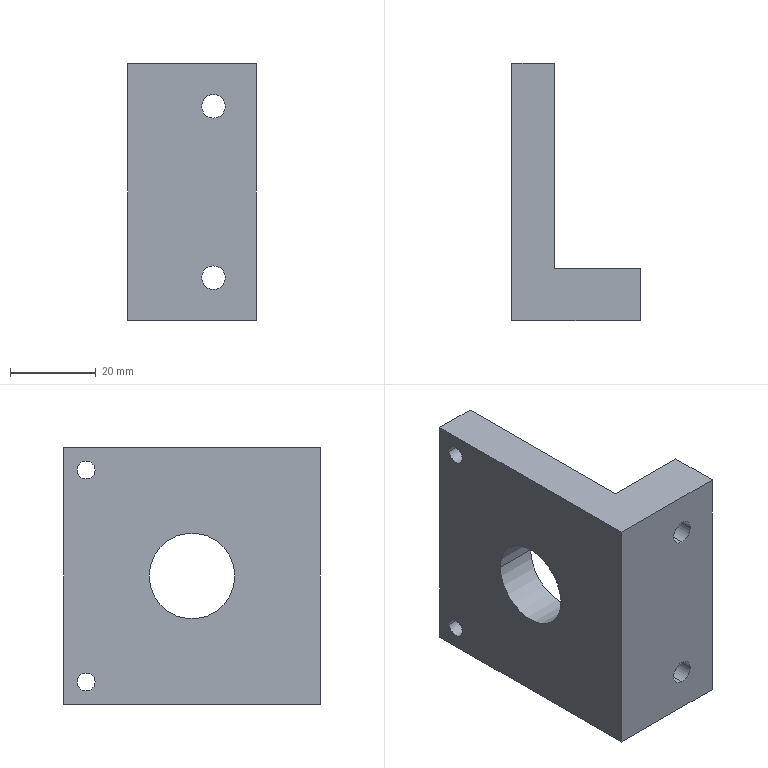Part | SolidWorks | features ICE 4, Extrusion 1 | 1 solid | 24 faces | box 30 x 60 x 60 mm | volume 45776 mm3 | cylinder 14 | plane 10 | commonest cylinder face diameters 4.2 x4 5.5 x4 10 x4 20 x2
STEP:
#1=CARTESIAN_POINT('',(-2.892,-8.477,45.));
#2=VERTEX_POINT('',#1);
#3=CARTESIAN_POINT('',(-2.892,-8.477,55.));
#4=VERTEX_POINT('',#3);
#5=CARTESIAN_POINT('',(-2.892,-8.477,50.));
#6=DIRECTION('',(0.,1.,0.));
#7=DIRECTION('',(0.,0.,1.));
#8=AXIS2_PLACEMENT_3D('',#5,#6,#7);
#9=CIRCLE('',#8,5.);
#10=EDGE_CURVE('',#2,#4,#9,.T.);
#11=ORIENTED_EDGE('',*,*,#10,.F.);
#12=CARTESIAN_POINT('',(-2.892,-2.677,45.));
#13=VERTEX_POINT('',#12);
#14=CARTESIAN_POINT('',(-2.892,-8.477,45.));
#15=DIRECTION('',(0.,1.,0.));
#16=VECTOR('',#15,1000.);
#17=LINE('',#14,#16);
#18=EDGE_CURVE('',#2,#13,#17,.T.);
#19=ORIENTED_EDGE('',*,*,#18,.T.);
#20=CARTESIAN_POINT('',(-2.892,-2.677,55.));
#21=VERTEX_POINT('',#20);
#22=CARTESIAN_POINT('',(-2.892,-2.677,50.));
#23=DIRECTION('',(0.,1.,0.));
#24=DIRECTION('',(0.,0.,1.));
#25=AXIS2_PLACEMENT_3D('',#22,#23,#24);
#26=CIRCLE('',#25,5.);
#27=EDGE_CURVE('',#13,#21,#26,.T.);
#28=ORIENTED_EDGE('',*,*,#27,.T.);
#29=CARTESIAN_POINT('',(-2.892,-8.477,55.));
#30=DIRECTION('',(0.,1.,0.));
#31=VECTOR('',#30,1000.);
#32=LINE('',#29,#31);
#33=EDGE_CURVE('',#4,#21,#32,.T.);
#34=ORIENTED_EDGE('',*,*,#33,.F.);
#35=EDGE_LOOP('',(#11,#19,#28,#34));
#36=FACE_OUTER_BOUND('',#35,.T.);
#37=CARTESIAN_POINT('',(-2.892,-8.477,50.));
#38=DIRECTION('',(0.,1.,0.));
#39=DIRECTION('',(0.,0.,1.));
#40=AXIS2_PLACEMENT_3D('',#37,#38,#39);
#41=CYLINDRICAL_SURFACE('',#40,5.);
#42=ADVANCED_FACE('',(#36),#41,.F.);
#43=CARTESIAN_POINT('',(-2.892,-8.477,5.));
#44=VERTEX_POINT('',#43);
#45=CARTESIAN_POINT('',(-2.892,-8.477,15.));
#46=VERTEX_POINT('',#45);
#47=CARTESIAN_POINT('',(-2.892,-8.477,10.));
#48=DIRECTION('',(0.,1.,0.));
#49=DIRECTION('',(0.,0.,1.));
#50=AXIS2_PLACEMENT_3D('',#47,#48,#49);
#51=CIRCLE('',#50,5.);
#52=EDGE_CURVE('',#44,#46,#51,.T.);
#53=ORIENTED_EDGE('',*,*,#52,.F.);
#54=CARTESIAN_POINT('',(-2.892,-2.677,5.));
#55=VERTEX_POINT('',#54);
#56=CARTESIAN_POINT('',(-2.892,-8.477,5.));
#57=DIRECTION('',(0.,1.,0.));
#58=VECTOR('',#57,1000.);
#59=LINE('',#56,#58);
#60=EDGE_CURVE('',#44,#55,#59,.T.);
#61=ORIENTED_EDGE('',*,*,#60,.T.);
#62=CARTESIAN_POINT('',(-2.892,-2.677,15.));
#63=VERTEX_POINT('',#62);
#64=CARTESIAN_POINT('',(-2.892,-2.677,10.));
#65=DIRECTION('',(0.,1.,0.));
#66=DIRECTION('',(0.,0.,1.));
#67=AXIS2_PLACEMENT_3D('',#64,#65,#66);
#68=CIRCLE('',#67,5.);
#69=EDGE_CURVE('',#55,#63,#68,.T.);
#70=ORIENTED_EDGE('',*,*,#69,.T.);
#71=CARTESIAN_POINT('',(-2.892,-8.477,15.));
#72=DIRECTION('',(0.,1.,0.));
#73=VECTOR('',#72,1000.);
#74=LINE('',#71,#73);
#75=EDGE_CURVE('',#46,#63,#74,.T.);
#76=ORIENTED_EDGE('',*,*,#75,.F.);
#77=EDGE_LOOP('',(#53,#61,#70,#76));
#78=FACE_OUTER_BOUND('',#77,.T.);
#79=CARTESIAN_POINT('',(-2.892,-8.477,10.));
#80=DIRECTION('',(0.,1.,0.));
#81=DIRECTION('',(0.,0.,1.));
#82=AXIS2_PLACEMENT_3D('',#79,#80,#81);
#83=CYLINDRICAL_SURFACE('',#82,5.);
#84=ADVANCED_FACE('',(#78),#83,.F.);
#85=CARTESIAN_POINT('',(-22.892,37.973,54.75));
#86=VERTEX_POINT('',#85);
#87=CARTESIAN_POINT('',(-22.892,42.173,54.75));
#88=VERTEX_POINT('',#87);
#89=CARTESIAN_POINT('',(-22.892,40.073,54.75));
#90=DIRECTION('',(1.,0.,0.));
#91=DIRECTION('',(0.,1.,0.));
#92=AXIS2_PLACEMENT_3D('',#89,#90,#91);
#93=CIRCLE('',#92,2.1);
#94=EDGE_CURVE('',#86,#88,#93,.T.);
#95=ORIENTED_EDGE('',*,*,#94,.F.);
#96=CARTESIAN_POINT('',(-12.892,37.973,54.75));
#97=VERTEX_POINT('',#96);
#98=CARTESIAN_POINT('',(-22.892,37.973,54.75));
#99=DIRECTION('',(1.,0.,0.));
#100=VECTOR('',#99,1000.);
#101=LINE('',#98,#100);
#102=EDGE_CURVE('',#86,#97,#101,.T.);
#103=ORIENTED_EDGE('',*,*,#102,.T.);
#104=CARTESIAN_POINT('',(-12.892,42.173,54.75));
#105=VERTEX_POINT('',#104);
#106=CARTESIAN_POINT('',(-12.892,40.073,54.75));
#107=DIRECTION('',(1.,0.,0.));
#108=DIRECTION('',(0.,1.,0.));
#109=AXIS2_PLACEMENT_3D('',#106,#107,#108);
#110=CIRCLE('',#109,2.1);
#111=EDGE_CURVE('',#97,#105,#110,.T.);
#112=ORIENTED_EDGE('',*,*,#111,.T.);
#113=CARTESIAN_POINT('',(-22.892,42.173,54.75));
#114=DIRECTION('',(1.,0.,0.));
#115=VECTOR('',#114,1000.);
#116=LINE('',#113,#115);
#117=EDGE_CURVE('',#88,#105,#116,.T.);
#118=ORIENTED_EDGE('',*,*,#117,.F.);
#119=EDGE_LOOP('',(#95,#103,#112,#118));
#120=FACE_OUTER_BOUND('',#119,.T.);
#121=CARTESIAN_POINT('',(-22.892,40.073,54.75));
#122=DIRECTION('',(1.,0.,0.));
#123=DIRECTION('',(0.,1.,0.));
#124=AXIS2_PLACEMENT_3D('',#121,#122,#123);
#125=CYLINDRICAL_SURFACE('',#124,2.1);
#126=ADVANCED_FACE('',(#120),#125,.F.);
#127=CARTESIAN_POINT('',(-22.892,37.973,5.25));
#128=VERTEX_POINT('',#127);
#129=CARTESIAN_POINT('',(-22.892,42.173,5.25));
#130=VERTEX_POINT('',#129);
#131=CARTESIAN_POINT('',(-22.892,40.073,5.25));
#132=DIRECTION('',(1.,0.,0.));
#133=DIRECTION('',(0.,1.,0.));
#134=AXIS2_PLACEMENT_3D('',#131,#132,#133);
#135=CIRCLE('',#134,2.1);
#136=EDGE_CURVE('',#128,#130,#135,.T.);
#137=ORIENTED_EDGE('',*,*,#136,.F.);
#138=CARTESIAN_POINT('',(-12.892,37.973,5.25));
#139=VERTEX_POINT('',#138);
#140=CARTESIAN_POINT('',(-22.892,37.973,5.25));
#141=DIRECTION('',(1.,0.,0.));
#142=VECTOR('',#141,1000.);
#143=LINE('',#140,#142);
#144=EDGE_CURVE('',#128,#139,#143,.T.);
#145=ORIENTED_EDGE('',*,*,#144,.T.);
#146=CARTESIAN_POINT('',(-12.892,42.173,5.25));
#147=VERTEX_POINT('',#146);
#148=CARTESIAN_POINT('',(-12.892,40.073,5.25));
#149=DIRECTION('',(1.,0.,0.));
#150=DIRECTION('',(0.,1.,0.));
#151=AXIS2_PLACEMENT_3D('',#148,#149,#150);
#152=CIRCLE('',#151,2.1);
#153=EDGE_CURVE('',#139,#147,#152,.T.);
#154=ORIENTED_EDGE('',*,*,#153,.T.);
#155=CARTESIAN_POINT('',(-22.892,42.173,5.25));
#156=DIRECTION('',(1.,0.,0.));
#157=VECTOR('',#156,1000.);
#158=LINE('',#155,#157);
#159=EDGE_CURVE('',#130,#147,#158,.T.);
#160=ORIENTED_EDGE('',*,*,#159,.F.);
#161=EDGE_LOOP('',(#137,#145,#154,#160));
#162=FACE_OUTER_BOUND('',#161,.T.);
#163=CARTESIAN_POINT('',(-22.892,40.073,5.25));
#164=DIRECTION('',(1.,0.,0.));
#165=DIRECTION('',(0.,1.,0.));
#166=AXIS2_PLACEMENT_3D('',#163,#164,#165);
#167=CYLINDRICAL_SURFACE('',#166,2.1);
#168=ADVANCED_FACE('',(#162),#167,.F.);
#169=CARTESIAN_POINT('',(-22.892,5.323,30.));
#170=VERTEX_POINT('',#169);
#171=CARTESIAN_POINT('',(-22.892,25.323,30.));
#172=VERTEX_POINT('',#171);
#173=CARTESIAN_POINT('',(-22.892,15.323,30.));
#174=DIRECTION('',(1.,0.,0.));
#175=DIRECTION('',(0.,1.,0.));
#176=AXIS2_PLACEMENT_3D('',#173,#174,#175);
#177=CIRCLE('',#176,10.);
#178=EDGE_CURVE('',#170,#172,#177,.T.);
#179=ORIENTED_EDGE('',*,*,#178,.F.);
#180=CARTESIAN_POINT('',(-12.892,5.323,30.));
#181=VERTEX_POINT('',#180);
#182=CARTESIAN_POINT('',(-22.892,5.323,30.));
#183=DIRECTION('',(1.,0.,0.));
#184=VECTOR('',#183,1000.);
#185=LINE('',#182,#184);
#186=EDGE_CURVE('',#170,#181,#185,.T.);
#187=ORIENTED_EDGE('',*,*,#186,.T.);
#188=CARTESIAN_POINT('',(-12.892,25.323,30.));
#189=VERTEX_POINT('',#188);
#190=CARTESIAN_POINT('',(-12.892,15.323,30.));
#191=DIRECTION('',(1.,0.,0.));
#192=DIRECTION('',(0.,1.,0.));
#193=AXIS2_PLACEMENT_3D('',#190,#191,#192);
#194=CIRCLE('',#193,10.);
#195=EDGE_CURVE('',#181,#189,#194,.T.);
#196=ORIENTED_EDGE('',*,*,#195,.T.);
#197=CARTESIAN_POINT('',(-22.892,25.323,30.));
#198=DIRECTION('',(1.,0.,0.));
#199=VECTOR('',#198,1000.);
#200=LINE('',#197,#199);
#201=EDGE_CURVE('',#172,#189,#200,.T.);
#202=ORIENTED_EDGE('',*,*,#201,.F.);
#203=EDGE_LOOP('',(#179,#187,#196,#202));
#204=FACE_OUTER_BOUND('',#203,.T.);
#205=CARTESIAN_POINT('',(-22.892,15.323,30.));
#206=DIRECTION('',(1.,0.,0.));
#207=DIRECTION('',(0.,1.,0.));
#208=AXIS2_PLACEMENT_3D('',#205,#206,#207);
#209=CYLINDRICAL_SURFACE('',#208,10.);
#210=ADVANCED_FACE('',(#204),#209,.F.);
#211=CARTESIAN_POINT('',(-2.892,-14.677,7.25));
#212=VERTEX_POINT('',#211);
#213=CARTESIAN_POINT('',(-2.892,-14.677,12.75));
#214=VERTEX_POINT('',#213);
#215=CARTESIAN_POINT('',(-2.892,-14.677,10.));
#216=DIRECTION('',(0.,1.,0.));
#217=DIRECTION('',(0.,0.,1.));
#218=AXIS2_PLACEMENT_3D('',#215,#216,#217);
#219=CIRCLE('',#218,2.75);
#220=EDGE_CURVE('',#212,#214,#219,.T.);
#221=ORIENTED_EDGE('',*,*,#220,.F.);
#222=CARTESIAN_POINT('',(-2.892,-8.477,7.25));
#223=VERTEX_POINT('',#222);
#224=CARTESIAN_POINT('',(-2.892,-14.677,7.25));
#225=DIRECTION('',(0.,1.,0.));
#226=VECTOR('',#225,1000.);
#227=LINE('',#224,#226);
#228=EDGE_CURVE('',#212,#223,#227,.T.);
#229=ORIENTED_EDGE('',*,*,#228,.T.);
#230=CARTESIAN_POINT('',(-2.892,-8.477,12.75));
#231=VERTEX_POINT('',#230);
#232=CARTESIAN_POINT('',(-2.892,-8.477,10.));
#233=DIRECTION('',(0.,-1.,0.));
#234=DIRECTION('',(0.,0.,1.));
#235=AXIS2_PLACEMENT_3D('',#232,#233,#234);
#236=CIRCLE('',#235,2.75);
#237=EDGE_CURVE('',#231,#223,#236,.T.);
#238=ORIENTED_EDGE('',*,*,#237,.F.);
#239=CARTESIAN_POINT('',(-2.892,-14.677,12.75));
#240=DIRECTION('',(0.,1.,0.));
#241=VECTOR('',#240,1000.);
#242=LINE('',#239,#241);
#243=EDGE_CURVE('',#214,#231,#242,.T.);
#244=ORIENTED_EDGE('',*,*,#243,.F.);
#245=EDGE_LOOP('',(#221,#229,#238,#244));
#246=FACE_OUTER_BOUND('',#245,.T.);
#247=CARTESIAN_POINT('',(-2.892,-14.677,10.));
#248=DIRECTION('',(0.,1.,0.));
#249=DIRECTION('',(0.,0.,1.));
#250=AXIS2_PLACEMENT_3D('',#247,#248,#249);
#251=CYLINDRICAL_SURFACE('',#250,2.75);
#252=ADVANCED_FACE('',(#246),#251,.F.);
#253=CARTESIAN_POINT('',(-2.892,-14.677,47.25));
#254=VERTEX_POINT('',#253);
#255=CARTESIAN_POINT('',(-2.892,-14.677,52.75));
#256=VERTEX_POINT('',#255);
#257=CARTESIAN_POINT('',(-2.892,-14.677,50.));
#258=DIRECTION('',(0.,1.,0.));
#259=DIRECTION('',(0.,0.,1.));
#260=AXIS2_PLACEMENT_3D('',#257,#258,#259);
#261=CIRCLE('',#260,2.75);
#262=EDGE_CURVE('',#254,#256,#261,.T.);
#263=ORIENTED_EDGE('',*,*,#262,.F.);
#264=CARTESIAN_POINT('',(-2.892,-8.477,47.25));
#265=VERTEX_POINT('',#264);
#266=CARTESIAN_POINT('',(-2.892,-14.677,47.25));
#267=DIRECTION('',(0.,1.,0.));
#268=VECTOR('',#267,1000.);
#269=LINE('',#266,#268);
#270=EDGE_CURVE('',#254,#265,#269,.T.);
#271=ORIENTED_EDGE('',*,*,#270,.T.);
#272=CARTESIAN_POINT('',(-2.892,-8.477,52.75));
#273=VERTEX_POINT('',#272);
#274=CARTESIAN_POINT('',(-2.892,-8.477,50.));
#275=DIRECTION('',(0.,-1.,0.));
#276=DIRECTION('',(0.,0.,1.));
#277=AXIS2_PLACEMENT_3D('',#274,#275,#276);
#278=CIRCLE('',#277,2.75);
#279=EDGE_CURVE('',#273,#265,#278,.T.);
#280=ORIENTED_EDGE('',*,*,#279,.F.);
#281=CARTESIAN_POINT('',(-2.892,-14.677,52.75));
#282=DIRECTION('',(0.,1.,0.));
#283=VECTOR('',#282,1000.);
#284=LINE('',#281,#283);
#285=EDGE_CURVE('',#256,#273,#284,.T.);
#286=ORIENTED_EDGE('',*,*,#285,.F.);
#287=EDGE_LOOP('',(#263,#271,#280,#286));
#288=FACE_OUTER_BOUND('',#287,.T.);
#289=CARTESIAN_POINT('',(-2.892,-14.677,50.));
#290=DIRECTION('',(0.,1.,0.));
#291=DIRECTION('',(0.,0.,1.));
#292=AXIS2_PLACEMENT_3D('',#289,#290,#291);
#293=CYLINDRICAL_SURFACE('',#292,2.75);
#294=ADVANCED_FACE('',(#288),#293,.F.);
#295=ORIENTED_EDGE('',*,*,#270,.F.);
#296=CARTESIAN_POINT('',(-2.892,-14.677,50.));
#297=DIRECTION('',(0.,1.,0.));
#298=DIRECTION('',(0.,0.,1.));
#299=AXIS2_PLACEMENT_3D('',#296,#297,#298);
#300=CIRCLE('',#299,2.75);
#301=EDGE_CURVE('',#256,#254,#300,.T.);
#302=ORIENTED_EDGE('',*,*,#301,.F.);
#303=ORIENTED_EDGE('',*,*,#285,.T.);
#304=CARTESIAN_POINT('',(-2.892,-8.477,50.));
#305=DIRECTION('',(0.,-1.,0.));
#306=DIRECTION('',(0.,0.,1.));
#307=AXIS2_PLACEMENT_3D('',#304,#305,#306);
#308=CIRCLE('',#307,2.75);
#309=EDGE_CURVE('',#265,#273,#308,.T.);
#310=ORIENTED_EDGE('',*,*,#309,.F.);
#311=EDGE_LOOP('',(#295,#302,#303,#310));
#312=FACE_OUTER_BOUND('',#311,.T.);
#313=CARTESIAN_POINT('',(-2.892,-14.677,50.));
#314=DIRECTION('',(0.,1.,0.));
#315=DIRECTION('',(0.,0.,1.));
#316=AXIS2_PLACEMENT_3D('',#313,#314,#315);
#317=CYLINDRICAL_SURFACE('',#316,2.75);
#318=ADVANCED_FACE('',(#312),#317,.F.);
#319=ORIENTED_EDGE('',*,*,#228,.F.);
#320=CARTESIAN_POINT('',(-2.892,-14.677,10.));
#321=DIRECTION('',(0.,1.,0.));
#322=DIRECTION('',(0.,0.,1.));
#323=AXIS2_PLACEMENT_3D('',#320,#321,#322);
#324=CIRCLE('',#323,2.75);
#325=EDGE_CURVE('',#214,#212,#324,.T.);
#326=ORIENTED_EDGE('',*,*,#325,.F.);
#327=ORIENTED_EDGE('',*,*,#243,.T.);
#328=CARTESIAN_POINT('',(-2.892,-8.477,10.));
#329=DIRECTION('',(0.,-1.,0.));
#330=DIRECTION('',(0.,0.,1.));
#331=AXIS2_PLACEMENT_3D('',#328,#329,#330);
#332=CIRCLE('',#331,2.75);
#333=EDGE_CURVE('',#223,#231,#332,.T.);
#334=ORIENTED_EDGE('',*,*,#333,.F.);
#335=EDGE_LOOP('',(#319,#326,#327,#334));
#336=FACE_OUTER_BOUND('',#335,.T.);
#337=CARTESIAN_POINT('',(-2.892,-14.677,10.));
#338=DIRECTION('',(0.,1.,0.));
#339=DIRECTION('',(0.,0.,1.));
#340=AXIS2_PLACEMENT_3D('',#337,#338,#339);
#341=CYLINDRICAL_SURFACE('',#340,2.75);
#342=ADVANCED_FACE('',(#336),#341,.F.);
#343=CARTESIAN_POINT('',(-12.892,45.323,0.));
#344=VERTEX_POINT('',#343);
#345=CARTESIAN_POINT('',(-22.892,45.323,0.));
#346=VERTEX_POINT('',#345);
#347=CARTESIAN_POINT('',(-22.892,45.323,0.));
#348=DIRECTION('',(-1.,0.,0.));
#349=VECTOR('',#348,1000.);
#350=LINE('',#347,#349);
#351=EDGE_CURVE('',#344,#346,#350,.T.);
#352=ORIENTED_EDGE('',*,*,#351,.T.);
#353=CARTESIAN_POINT('',(-22.892,45.323,60.));
#354=VERTEX_POINT('',#353);
#355=CARTESIAN_POINT('',(-22.892,45.323,60.));
#356=DIRECTION('',(0.,0.,-1.));
#357=VECTOR('',#356,1000.);
#358=LINE('',#355,#357);
#359=EDGE_CURVE('',#354,#346,#358,.T.);
#360=ORIENTED_EDGE('',*,*,#359,.F.);
#361=CARTESIAN_POINT('',(-12.892,45.323,60.));
#362=VERTEX_POINT('',#361);
#363=CARTESIAN_POINT('',(-22.892,45.323,60.));
#364=DIRECTION('',(-1.,0.,0.));
#365=VECTOR('',#364,1000.);
#366=LINE('',#363,#365);
#367=EDGE_CURVE('',#362,#354,#366,.T.);
#368=ORIENTED_EDGE('',*,*,#367,.F.);
#369=CARTESIAN_POINT('',(-12.892,45.323,60.));
#370=DIRECTION('',(0.,0.,-1.));
#371=VECTOR('',#370,1000.);
#372=LINE('',#369,#371);
#373=EDGE_CURVE('',#362,#344,#372,.T.);
#374=ORIENTED_EDGE('',*,*,#373,.T.);
#375=EDGE_LOOP('',(#352,#360,#368,#374));
#376=FACE_OUTER_BOUND('',#375,.T.);
#377=CARTESIAN_POINT('',(-22.892,45.323,60.));
#378=DIRECTION('',(0.,-1.,0.));
#379=DIRECTION('',(0.,0.,-1.));
#380=AXIS2_PLACEMENT_3D('',#377,#378,#379);
#381=PLANE('',#380);
#382=ADVANCED_FACE('',(#376),#381,.F.);
#383=CARTESIAN_POINT('',(-22.892,40.073,54.75));
#384=DIRECTION('',(1.,0.,0.));
#385=DIRECTION('',(0.,1.,0.));
#386=AXIS2_PLACEMENT_3D('',#383,#384,#385);
#387=CIRCLE('',#386,2.1);
#388=EDGE_CURVE('',#88,#86,#387,.T.);
#389=ORIENTED_EDGE('',*,*,#388,.T.);
#390=ORIENTED_EDGE('',*,*,#94,.T.);
#391=EDGE_LOOP('',(#389,#390));
#392=FACE_BOUND('',#391,.T.);
#393=CARTESIAN_POINT('',(-22.892,40.073,5.25));
#394=DIRECTION('',(1.,0.,0.));
#395=DIRECTION('',(0.,1.,0.));
#396=AXIS2_PLACEMENT_3D('',#393,#394,#395);
#397=CIRCLE('',#396,2.1);
#398=EDGE_CURVE('',#130,#128,#397,.T.);
#399=ORIENTED_EDGE('',*,*,#398,.T.);
#400=ORIENTED_EDGE('',*,*,#136,.T.);
#401=EDGE_LOOP('',(#399,#400));
#402=FACE_BOUND('',#401,.T.);
#403=CARTESIAN_POINT('',(-22.892,15.323,30.));
#404=DIRECTION('',(1.,0.,0.));
#405=DIRECTION('',(0.,1.,0.));
#406=AXIS2_PLACEMENT_3D('',#403,#404,#405);
#407=CIRCLE('',#406,10.);
#408=EDGE_CURVE('',#172,#170,#407,.T.);
#409=ORIENTED_EDGE('',*,*,#408,.T.);
#410=ORIENTED_EDGE('',*,*,#178,.T.);
#411=EDGE_LOOP('',(#409,#410));
#412=FACE_BOUND('',#411,.T.);
#413=CARTESIAN_POINT('',(-22.892,-14.677,0.));
#414=VERTEX_POINT('',#413);
#415=CARTESIAN_POINT('',(-22.892,-14.677,0.));
#416=DIRECTION('',(0.,-1.,0.));
#417=VECTOR('',#416,1000.);
#418=LINE('',#415,#417);
#419=EDGE_CURVE('',#346,#414,#418,.T.);
#420=ORIENTED_EDGE('',*,*,#419,.T.);
#421=CARTESIAN_POINT('',(-22.892,-14.677,60.));
#422=VERTEX_POINT('',#421);
#423=CARTESIAN_POINT('',(-22.892,-14.677,60.));
#424=DIRECTION('',(0.,0.,-1.));
#425=VECTOR('',#424,1000.);
#426=LINE('',#423,#425);
#427=EDGE_CURVE('',#422,#414,#426,.T.);
#428=ORIENTED_EDGE('',*,*,#427,.F.);
#429=CARTESIAN_POINT('',(-22.892,-14.677,60.));
#430=DIRECTION('',(0.,-1.,0.));
#431=VECTOR('',#430,1000.);
#432=LINE('',#429,#431);
#433=EDGE_CURVE('',#354,#422,#432,.T.);
#434=ORIENTED_EDGE('',*,*,#433,.F.);
#435=ORIENTED_EDGE('',*,*,#359,.T.);
#436=EDGE_LOOP('',(#420,#428,#434,#435));
#437=FACE_OUTER_BOUND('',#436,.T.);
#438=CARTESIAN_POINT('',(-22.892,-14.677,60.));
#439=DIRECTION('',(1.,0.,0.));
#440=DIRECTION('',(0.,0.,-1.));
#441=AXIS2_PLACEMENT_3D('',#438,#439,#440);
#442=PLANE('',#441);
#443=ADVANCED_FACE('',(#392,#402,#412,#437),#442,.F.);
#444=ORIENTED_EDGE('',*,*,#325,.T.);
#445=ORIENTED_EDGE('',*,*,#220,.T.);
#446=EDGE_LOOP('',(#444,#445));
#447=FACE_BOUND('',#446,.T.);
#448=ORIENTED_EDGE('',*,*,#301,.T.);
#449=ORIENTED_EDGE('',*,*,#262,.T.);
#450=EDGE_LOOP('',(#448,#449));
#451=FACE_BOUND('',#450,.T.);
#452=CARTESIAN_POINT('',(7.108,-14.677,0.));
#453=VERTEX_POINT('',#452);
#454=CARTESIAN_POINT('',(7.108,-14.677,0.));
#455=DIRECTION('',(1.,0.,0.));
#456=VECTOR('',#455,1000.);
#457=LINE('',#454,#456);
#458=EDGE_CURVE('',#414,#453,#457,.T.);
#459=ORIENTED_EDGE('',*,*,#458,.T.);
#460=CARTESIAN_POINT('',(7.108,-14.677,60.));
#461=VERTEX_POINT('',#460);
#462=CARTESIAN_POINT('',(7.108,-14.677,60.));
#463=DIRECTION('',(0.,0.,-1.));
#464=VECTOR('',#463,1000.);
#465=LINE('',#462,#464);
#466=EDGE_CURVE('',#461,#453,#465,.T.);
#467=ORIENTED_EDGE('',*,*,#466,.F.);
#468=CARTESIAN_POINT('',(7.108,-14.677,60.));
#469=DIRECTION('',(1.,0.,0.));
#470=VECTOR('',#469,1000.);
#471=LINE('',#468,#470);
#472=EDGE_CURVE('',#422,#461,#471,.T.);
#473=ORIENTED_EDGE('',*,*,#472,.F.);
#474=ORIENTED_EDGE('',*,*,#427,.T.);
#475=EDGE_LOOP('',(#459,#467,#473,#474));
#476=FACE_OUTER_BOUND('',#475,.T.);
#477=CARTESIAN_POINT('',(7.108,-14.677,60.));
#478=DIRECTION('',(0.,1.,0.));
#479=DIRECTION('',(-1.,0.,0.));
#480=AXIS2_PLACEMENT_3D('',#477,#478,#479);
#481=PLANE('',#480);
#482=ADVANCED_FACE('',(#447,#451,#476),#481,.F.);
#483=CARTESIAN_POINT('',(7.108,-2.677,0.));
#484=VERTEX_POINT('',#483);
#485=CARTESIAN_POINT('',(7.108,-2.677,0.));
#486=DIRECTION('',(0.,1.,0.));
#487=VECTOR('',#486,1000.);
#488=LINE('',#485,#487);
#489=EDGE_CURVE('',#453,#484,#488,.T.);
#490=ORIENTED_EDGE('',*,*,#489,.T.);
#491=CARTESIAN_POINT('',(7.108,-2.677,60.));
#492=VERTEX_POINT('',#491);
#493=CARTESIAN_POINT('',(7.108,-2.677,60.));
#494=DIRECTION('',(0.,0.,-1.));
#495=VECTOR('',#494,1000.);
#496=LINE('',#493,#495);
#497=EDGE_CURVE('',#492,#484,#496,.T.);
#498=ORIENTED_EDGE('',*,*,#497,.F.);
#499=CARTESIAN_POINT('',(7.108,-2.677,60.));
#500=DIRECTION('',(0.,1.,0.));
#501=VECTOR('',#500,1000.);
#502=LINE('',#499,#501);
#503=EDGE_CURVE('',#461,#492,#502,.T.);
#504=ORIENTED_EDGE('',*,*,#503,.F.);
#505=ORIENTED_EDGE('',*,*,#466,.T.);
#506=EDGE_LOOP('',(#490,#498,#504,#505));
#507=FACE_OUTER_BOUND('',#506,.T.);
#508=CARTESIAN_POINT('',(7.108,-2.677,60.));
#509=DIRECTION('',(-1.,0.,0.));
#510=DIRECTION('',(0.,-1.,0.));
#511=AXIS2_PLACEMENT_3D('',#508,#509,#510);
#512=PLANE('',#511);
#513=ADVANCED_FACE('',(#507),#512,.F.);
#514=CARTESIAN_POINT('',(-2.892,-2.677,10.));
#515=DIRECTION('',(0.,1.,0.));
#516=DIRECTION('',(0.,0.,1.));
#517=AXIS2_PLACEMENT_3D('',#514,#515,#516);
#518=CIRCLE('',#517,5.);
#519=EDGE_CURVE('',#63,#55,#518,.T.);
#520=ORIENTED_EDGE('',*,*,#519,.F.);
#521=ORIENTED_EDGE('',*,*,#69,.F.);
#522=EDGE_LOOP('',(#520,#521));
#523=FACE_BOUND('',#522,.T.);
#524=CARTESIAN_POINT('',(-2.892,-2.677,50.));
#525=DIRECTION('',(0.,1.,0.));
#526=DIRECTION('',(0.,0.,1.));
#527=AXIS2_PLACEMENT_3D('',#524,#525,#526);
#528=CIRCLE('',#527,5.);
#529=EDGE_CURVE('',#21,#13,#528,.T.);
#530=ORIENTED_EDGE('',*,*,#529,.F.);
#531=ORIENTED_EDGE('',*,*,#27,.F.);
#532=EDGE_LOOP('',(#530,#531));
#533=FACE_BOUND('',#532,.T.);
#534=CARTESIAN_POINT('',(-12.892,-2.677,0.));
#535=VERTEX_POINT('',#534);
#536=CARTESIAN_POINT('',(-12.892,-2.677,0.));
#537=DIRECTION('',(-1.,0.,0.));
#538=VECTOR('',#537,1000.);
#539=LINE('',#536,#538);
#540=EDGE_CURVE('',#484,#535,#539,.T.);
#541=ORIENTED_EDGE('',*,*,#540,.T.);
#542=CARTESIAN_POINT('',(-12.892,-2.677,60.));
#543=VERTEX_POINT('',#542);
#544=CARTESIAN_POINT('',(-12.892,-2.677,60.));
#545=DIRECTION('',(0.,0.,-1.));
#546=VECTOR('',#545,1000.);
#547=LINE('',#544,#546);
#548=EDGE_CURVE('',#543,#535,#547,.T.);
#549=ORIENTED_EDGE('',*,*,#548,.F.);
#550=CARTESIAN_POINT('',(-12.892,-2.677,60.));
#551=DIRECTION('',(-1.,0.,0.));
#552=VECTOR('',#551,1000.);
#553=LINE('',#550,#552);
#554=EDGE_CURVE('',#492,#543,#553,.T.);
#555=ORIENTED_EDGE('',*,*,#554,.F.);
#556=ORIENTED_EDGE('',*,*,#497,.T.);
#557=EDGE_LOOP('',(#541,#549,#555,#556));
#558=FACE_OUTER_BOUND('',#557,.T.);
#559=CARTESIAN_POINT('',(-12.892,-2.677,60.));
#560=DIRECTION('',(0.,-1.,0.));
#561=DIRECTION('',(0.,0.,-1.));
#562=AXIS2_PLACEMENT_3D('',#559,#560,#561);
#563=PLANE('',#562);
#564=ADVANCED_FACE('',(#523,#533,#558),#563,.F.);
#565=CARTESIAN_POINT('',(-12.892,40.073,54.75));
#566=DIRECTION('',(1.,0.,0.));
#567=DIRECTION('',(0.,1.,0.));
#568=AXIS2_PLACEMENT_3D('',#565,#566,#567);
#569=CIRCLE('',#568,2.1);
#570=EDGE_CURVE('',#105,#97,#569,.T.);
#571=ORIENTED_EDGE('',*,*,#570,.F.);
#572=ORIENTED_EDGE('',*,*,#111,.F.);
#573=EDGE_LOOP('',(#571,#572));
#574=FACE_BOUND('',#573,.T.);
#575=CARTESIAN_POINT('',(-12.892,40.073,5.25));
#576=DIRECTION('',(1.,0.,0.));
#577=DIRECTION('',(0.,1.,0.));
#578=AXIS2_PLACEMENT_3D('',#575,#576,#577);
#579=CIRCLE('',#578,2.1);
#580=EDGE_CURVE('',#147,#139,#579,.T.);
#581=ORIENTED_EDGE('',*,*,#580,.F.);
#582=ORIENTED_EDGE('',*,*,#153,.F.);
#583=EDGE_LOOP('',(#581,#582));
#584=FACE_BOUND('',#583,.T.);
#585=CARTESIAN_POINT('',(-12.892,15.323,30.));
#586=DIRECTION('',(1.,0.,0.));
#587=DIRECTION('',(0.,1.,0.));
#588=AXIS2_PLACEMENT_3D('',#585,#586,#587);
#589=CIRCLE('',#588,10.);
#590=EDGE_CURVE('',#189,#181,#589,.T.);
#591=ORIENTED_EDGE('',*,*,#590,.F.);
#592=ORIENTED_EDGE('',*,*,#195,.F.);
#593=EDGE_LOOP('',(#591,#592));
#594=FACE_BOUND('',#593,.T.);
#595=CARTESIAN_POINT('',(-12.892,45.323,0.));
#596=DIRECTION('',(0.,1.,0.));
#597=VECTOR('',#596,1000.);
#598=LINE('',#595,#597);
#599=EDGE_CURVE('',#535,#344,#598,.T.);
#600=ORIENTED_EDGE('',*,*,#599,.T.);
#601=ORIENTED_EDGE('',*,*,#373,.F.);
#602=CARTESIAN_POINT('',(-12.892,45.323,60.));
#603=DIRECTION('',(0.,1.,0.));
#604=VECTOR('',#603,1000.);
#605=LINE('',#602,#604);
#606=EDGE_CURVE('',#543,#362,#605,.T.);
#607=ORIENTED_EDGE('',*,*,#606,.F.);
#608=ORIENTED_EDGE('',*,*,#548,.T.);
#609=EDGE_LOOP('',(#600,#601,#607,#608));
#610=FACE_OUTER_BOUND('',#609,.T.);
#611=CARTESIAN_POINT('',(-12.892,45.323,60.));
#612=DIRECTION('',(-1.,0.,0.));
#613=DIRECTION('',(0.,-1.,0.));
#614=AXIS2_PLACEMENT_3D('',#611,#612,#613);
#615=PLANE('',#614);
#616=ADVANCED_FACE('',(#574,#584,#594,#610),#615,.F.);
#617=ORIENTED_EDGE('',*,*,#367,.T.);
#618=ORIENTED_EDGE('',*,*,#433,.T.);
#619=ORIENTED_EDGE('',*,*,#472,.T.);
#620=ORIENTED_EDGE('',*,*,#503,.T.);
#621=ORIENTED_EDGE('',*,*,#554,.T.);
#622=ORIENTED_EDGE('',*,*,#606,.T.);
#623=EDGE_LOOP('',(#617,#618,#619,#620,#621,#622));
#624=FACE_OUTER_BOUND('',#623,.T.);
#625=CARTESIAN_POINT('',(0.,0.,60.));
#626=DIRECTION('',(0.,0.,-1.));
#627=DIRECTION('',(-1.,0.,0.));
#628=AXIS2_PLACEMENT_3D('',#625,#626,#627);
#629=PLANE('',#628);
#630=ADVANCED_FACE('',(#624),#629,.F.);
#631=ORIENTED_EDGE('',*,*,#351,.F.);
#632=ORIENTED_EDGE('',*,*,#599,.F.);
#633=ORIENTED_EDGE('',*,*,#540,.F.);
#634=ORIENTED_EDGE('',*,*,#489,.F.);
#635=ORIENTED_EDGE('',*,*,#458,.F.);
#636=ORIENTED_EDGE('',*,*,#419,.F.);
#637=EDGE_LOOP('',(#631,#632,#633,#634,#635,#636));
#638=FACE_OUTER_BOUND('',#637,.T.);
#639=CARTESIAN_POINT('',(0.,0.,0.));
#640=DIRECTION('',(0.,0.,-1.));
#641=DIRECTION('',(-1.,0.,0.));
#642=AXIS2_PLACEMENT_3D('',#639,#640,#641);
#643=PLANE('',#642);
#644=ADVANCED_FACE('',(#638),#643,.T.);
#645=ORIENTED_EDGE('',*,*,#186,.F.);
#646=ORIENTED_EDGE('',*,*,#408,.F.);
#647=ORIENTED_EDGE('',*,*,#201,.T.);
#648=ORIENTED_EDGE('',*,*,#590,.T.);
#649=EDGE_LOOP('',(#645,#646,#647,#648));
#650=FACE_OUTER_BOUND('',#649,.T.);
#651=CARTESIAN_POINT('',(-22.892,15.323,30.));
#652=DIRECTION('',(1.,0.,0.));
#653=DIRECTION('',(0.,1.,0.));
#654=AXIS2_PLACEMENT_3D('',#651,#652,#653);
#655=CYLINDRICAL_SURFACE('',#654,10.);
#656=ADVANCED_FACE('',(#650),#655,.F.);
#657=ORIENTED_EDGE('',*,*,#144,.F.);
#658=ORIENTED_EDGE('',*,*,#398,.F.);
#659=ORIENTED_EDGE('',*,*,#159,.T.);
#660=ORIENTED_EDGE('',*,*,#580,.T.);
#661=EDGE_LOOP('',(#657,#658,#659,#660));
#662=FACE_OUTER_BOUND('',#661,.T.);
#663=CARTESIAN_POINT('',(-22.892,40.073,5.25));
#664=DIRECTION('',(1.,0.,0.));
#665=DIRECTION('',(0.,1.,0.));
#666=AXIS2_PLACEMENT_3D('',#663,#664,#665);
#667=CYLINDRICAL_SURFACE('',#666,2.1);
#668=ADVANCED_FACE('',(#662),#667,.F.);
#669=ORIENTED_EDGE('',*,*,#102,.F.);
#670=ORIENTED_EDGE('',*,*,#388,.F.);
#671=ORIENTED_EDGE('',*,*,#117,.T.);
#672=ORIENTED_EDGE('',*,*,#570,.T.);
#673=EDGE_LOOP('',(#669,#670,#671,#672));
#674=FACE_OUTER_BOUND('',#673,.T.);
#675=CARTESIAN_POINT('',(-22.892,40.073,54.75));
#676=DIRECTION('',(1.,0.,0.));
#677=DIRECTION('',(0.,1.,0.));
#678=AXIS2_PLACEMENT_3D('',#675,#676,#677);
#679=CYLINDRICAL_SURFACE('',#678,2.1);
#680=ADVANCED_FACE('',(#674),#679,.F.);
#681=CARTESIAN_POINT('',(-2.892,-8.477,10.));
#682=DIRECTION('',(0.,1.,0.));
#683=DIRECTION('',(0.,0.,1.));
#684=AXIS2_PLACEMENT_3D('',#681,#682,#683);
#685=CIRCLE('',#684,5.);
#686=EDGE_CURVE('',#46,#44,#685,.T.);
#687=ORIENTED_EDGE('',*,*,#686,.T.);
#688=ORIENTED_EDGE('',*,*,#52,.T.);
#689=EDGE_LOOP('',(#687,#688));
#690=FACE_OUTER_BOUND('',#689,.T.);
#691=ORIENTED_EDGE('',*,*,#237,.T.);
#692=ORIENTED_EDGE('',*,*,#333,.T.);
#693=EDGE_LOOP('',(#691,#692));
#694=FACE_BOUND('',#693,.T.);
#695=CARTESIAN_POINT('',(-2.892,-8.477,10.));
#696=DIRECTION('',(0.,1.,0.));
#697=DIRECTION('',(0.,0.,1.));
#698=AXIS2_PLACEMENT_3D('',#695,#696,#697);
#699=PLANE('',#698);
#700=ADVANCED_FACE('',(#690,#694),#699,.T.);
#701=ORIENTED_EDGE('',*,*,#60,.F.);
#702=ORIENTED_EDGE('',*,*,#686,.F.);
#703=ORIENTED_EDGE('',*,*,#75,.T.);
#704=ORIENTED_EDGE('',*,*,#519,.T.);
#705=EDGE_LOOP('',(#701,#702,#703,#704));
#706=FACE_OUTER_BOUND('',#705,.T.);
#707=CARTESIAN_POINT('',(-2.892,-8.477,10.));
#708=DIRECTION('',(0.,1.,0.));
#709=DIRECTION('',(0.,0.,1.));
#710=AXIS2_PLACEMENT_3D('',#707,#708,#709);
#711=CYLINDRICAL_SURFACE('',#710,5.);
#712=ADVANCED_FACE('',(#706),#711,.F.);
#713=CARTESIAN_POINT('',(-2.892,-8.477,50.));
#714=DIRECTION('',(0.,1.,0.));
#715=DIRECTION('',(0.,0.,1.));
#716=AXIS2_PLACEMENT_3D('',#713,#714,#715);
#717=CIRCLE('',#716,5.);
#718=EDGE_CURVE('',#4,#2,#717,.T.);
#719=ORIENTED_EDGE('',*,*,#718,.T.);
#720=ORIENTED_EDGE('',*,*,#10,.T.);
#721=EDGE_LOOP('',(#719,#720));
#722=FACE_OUTER_BOUND('',#721,.T.);
#723=ORIENTED_EDGE('',*,*,#279,.T.);
#724=ORIENTED_EDGE('',*,*,#309,.T.);
#725=EDGE_LOOP('',(#723,#724));
#726=FACE_BOUND('',#725,.T.);
#727=CARTESIAN_POINT('',(-2.892,-8.477,50.));
#728=DIRECTION('',(0.,1.,0.));
#729=DIRECTION('',(0.,0.,1.));
#730=AXIS2_PLACEMENT_3D('',#727,#728,#729);
#731=PLANE('',#730);
#732=ADVANCED_FACE('',(#722,#726),#731,.T.);
#733=ORIENTED_EDGE('',*,*,#18,.F.);
#734=ORIENTED_EDGE('',*,*,#718,.F.);
#735=ORIENTED_EDGE('',*,*,#33,.T.);
#736=ORIENTED_EDGE('',*,*,#529,.T.);
#737=EDGE_LOOP('',(#733,#734,#735,#736));
#738=FACE_OUTER_BOUND('',#737,.T.);
#739=CARTESIAN_POINT('',(-2.892,-8.477,50.));
#740=DIRECTION('',(0.,1.,0.));
#741=DIRECTION('',(0.,0.,1.));
#742=AXIS2_PLACEMENT_3D('',#739,#740,#741);
#743=CYLINDRICAL_SURFACE('',#742,5.);
#744=ADVANCED_FACE('',(#738),#743,.F.);
#745=CLOSED_SHELL('',(#42,#84,#126,#168,#210,#252,#294,#318,#342,#382,#443,#482,#513,#564,#616,#630,#644,#656,#668,#680,#700,#712,#732,#744));
#746=MANIFOLD_SOLID_BREP('',#745);
#747=CARTESIAN_POINT('',(0.,0.,0.));
#748=DIRECTION('',(0.,0.,1.));
#749=DIRECTION('',(1.,0.,0.));
#750=AXIS2_PLACEMENT_3D('',#747,#748,#749);
#751=(LENGTH_UNIT()NAMED_UNIT(*)SI_UNIT(.MILLI.,.METRE.));
#752=UNCERTAINTY_MEASURE_WITH_UNIT(LENGTH_MEASURE(0.00001),#751,'','');
#753=(NAMED_UNIT(*)PLANE_ANGLE_UNIT()SI_UNIT($,.RADIAN.));
#754=(NAMED_UNIT(*)SI_UNIT($,.STERADIAN.)SOLID_ANGLE_UNIT());
#755=(GEOMETRIC_REPRESENTATION_CONTEXT(3)GLOBAL_UNCERTAINTY_ASSIGNED_CONTEXT((#752))GLOBAL_UNIT_ASSIGNED_CONTEXT((#751,#753,#754))REPRESENTATION_CONTEXT('',''));
#756=ADVANCED_BREP_SHAPE_REPRESENTATION('',(#746,#750),#755);